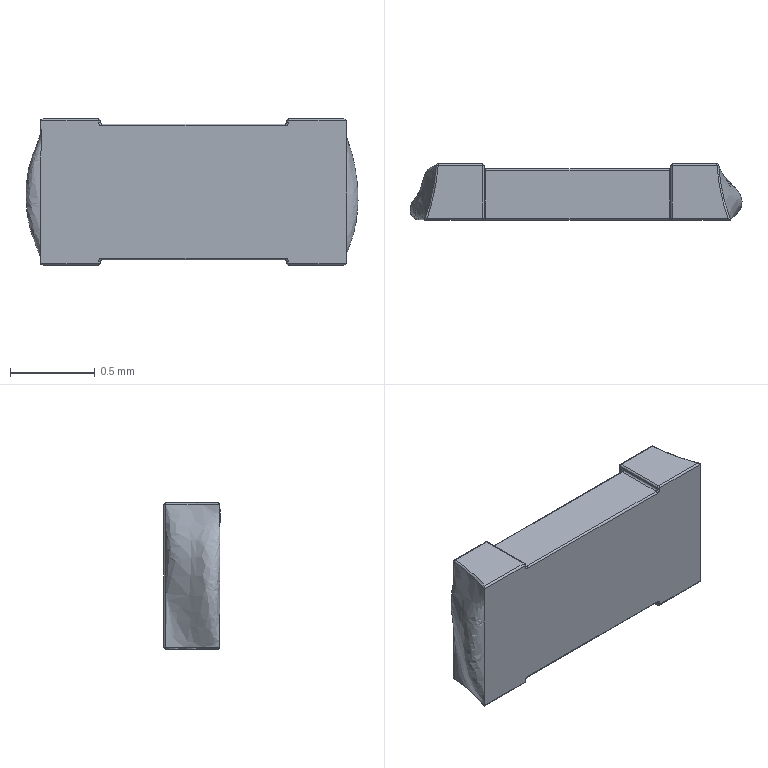Part | STEP file | NCP18XH103F03RB_1 | 1 solid | 68 faces | box 1.956 x 0.33 x 0.86 mm | volume 0.4616 mm3 | cylinder 30 | sphere 12 | torus 12 | plane 12 | spline 2 | commonest cylinder face diameters 0.02 x30